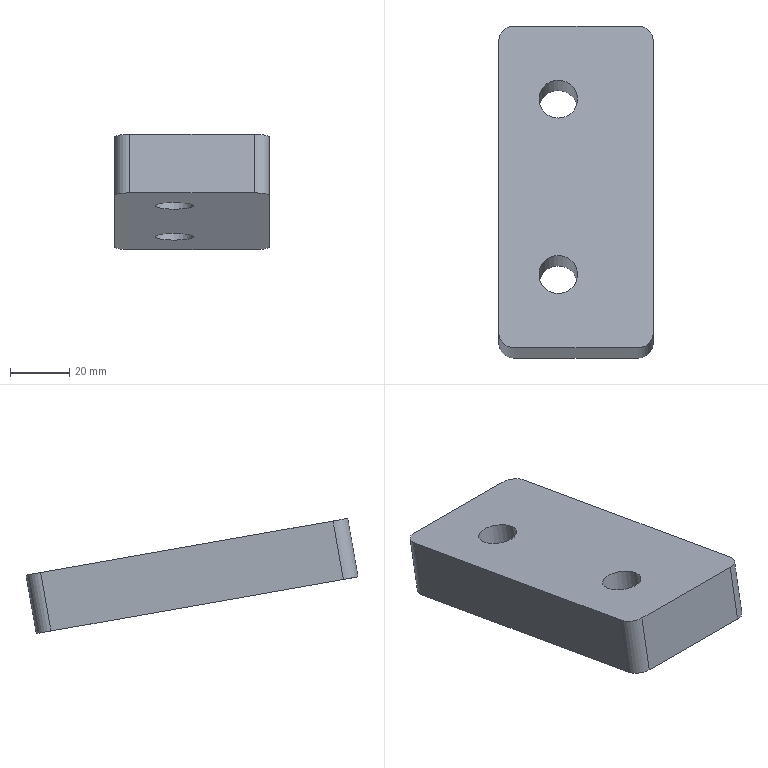Part | NX | features MAIN_BODY 2 | 1 solid | 12 faces | box 52 x 111.802 x 38.797 mm | volume 108662 mm3 | plane 6 | cylinder 6 | commonest cylinder face diameters 10 x4 13 x2
STEP:
#1=CARTESIAN_POINT('',(-1300.762,-795.713,-43.014));
#2=VERTEX_POINT('',#1);
#3=CARTESIAN_POINT('',(-1342.762,-795.713,-43.014));
#4=VERTEX_POINT('',#3);
#5=CARTESIAN_POINT('',(-1295.762,-795.713,-43.014));
#6=DIRECTION('',(-1.,0.,0.));
#7=VECTOR('',#6,1000.);
#8=LINE('',#5,#7);
#9=EDGE_CURVE('',#2,#4,#8,.T.);
#10=ORIENTED_EDGE('',*,*,#9,.T.);
#11=CARTESIAN_POINT('',(-1342.762,-792.24,-23.318));
#12=VERTEX_POINT('',#11);
#13=CARTESIAN_POINT('',(-1342.762,-792.24,-23.318));
#14=DIRECTION('',(0.,-0.1736,-0.9848));
#15=VECTOR('',#14,1000.);
#16=LINE('',#13,#15);
#17=EDGE_CURVE('',#12,#4,#16,.T.);
#18=ORIENTED_EDGE('',*,*,#17,.F.);
#19=CARTESIAN_POINT('',(-1300.762,-792.24,-23.318));
#20=VERTEX_POINT('',#19);
#21=CARTESIAN_POINT('',(-1295.762,-792.24,-23.318));
#22=DIRECTION('',(-1.,0.,0.));
#23=VECTOR('',#22,1000.);
#24=LINE('',#21,#23);
#25=EDGE_CURVE('',#20,#12,#24,.T.);
#26=ORIENTED_EDGE('',*,*,#25,.F.);
#27=CARTESIAN_POINT('',(-1300.762,-792.24,-23.318));
#28=DIRECTION('',(0.,-0.1736,-0.9848));
#29=VECTOR('',#28,1000.);
#30=LINE('',#27,#29);
#31=EDGE_CURVE('',#2,#20,#30,.F.);
#32=ORIENTED_EDGE('',*,*,#31,.F.);
#33=EDGE_LOOP('',(#10,#18,#26,#32));
#34=FACE_BOUND('',#33,.T.);
#35=CARTESIAN_POINT('',(-1295.762,-792.24,-23.318));
#36=DIRECTION('',(0.,0.9848,-0.1736));
#37=DIRECTION('',(1.,0.,0.));
#38=AXIS2_PLACEMENT_3D('',#35,#36,#37);
#39=PLANE('',#38);
#40=ADVANCED_FACE('',(#34),#39,.T.);
#41=CARTESIAN_POINT('',(-1347.762,-800.637,-42.145));
#42=VERTEX_POINT('',#41);
#43=CARTESIAN_POINT('',(-1347.762,-899.118,-24.781));
#44=VERTEX_POINT('',#43);
#45=CARTESIAN_POINT('',(-1347.762,-795.713,-43.014));
#46=DIRECTION('',(0.,-0.9848,0.1736));
#47=VECTOR('',#46,1000.);
#48=LINE('',#45,#47);
#49=EDGE_CURVE('',#42,#44,#48,.T.);
#50=ORIENTED_EDGE('',*,*,#49,.T.);
#51=CARTESIAN_POINT('',(-1347.762,-895.645,-5.085));
#52=VERTEX_POINT('',#51);
#53=CARTESIAN_POINT('',(-1347.762,-895.645,-5.085));
#54=DIRECTION('',(0.,-0.1736,-0.9848));
#55=VECTOR('',#54,1000.);
#56=LINE('',#53,#55);
#57=EDGE_CURVE('',#52,#44,#56,.T.);
#58=ORIENTED_EDGE('',*,*,#57,.F.);
#59=CARTESIAN_POINT('',(-1347.762,-797.164,-22.449));
#60=VERTEX_POINT('',#59);
#61=CARTESIAN_POINT('',(-1347.762,-792.24,-23.318));
#62=DIRECTION('',(0.,-0.9848,0.1736));
#63=VECTOR('',#62,1000.);
#64=LINE('',#61,#63);
#65=EDGE_CURVE('',#60,#52,#64,.T.);
#66=ORIENTED_EDGE('',*,*,#65,.F.);
#67=CARTESIAN_POINT('',(-1347.762,-797.164,-22.449));
#68=DIRECTION('',(0.,-0.1736,-0.9848));
#69=VECTOR('',#68,1000.);
#70=LINE('',#67,#69);
#71=EDGE_CURVE('',#42,#60,#70,.F.);
#72=ORIENTED_EDGE('',*,*,#71,.F.);
#73=EDGE_LOOP('',(#50,#58,#66,#72));
#74=FACE_BOUND('',#73,.T.);
#75=CARTESIAN_POINT('',(-1347.762,-792.24,-23.318));
#76=DIRECTION('',(-1.,0.,0.));
#77=DIRECTION('',(0.,0.9848,-0.1736));
#78=AXIS2_PLACEMENT_3D('',#75,#76,#77);
#79=PLANE('',#78);
#80=ADVANCED_FACE('',(#74),#79,.T.);
#81=CARTESIAN_POINT('',(-1295.762,-895.645,-5.085));
#82=VERTEX_POINT('',#81);
#83=CARTESIAN_POINT('',(-1295.762,-797.164,-22.449));
#84=VERTEX_POINT('',#83);
#85=CARTESIAN_POINT('',(-1295.762,-866.101,-10.294));
#86=DIRECTION('',(0.,0.9848,-0.1736));
#87=VECTOR('',#86,1000.);
#88=LINE('',#85,#87);
#89=EDGE_CURVE('',#82,#84,#88,.T.);
#90=ORIENTED_EDGE('',*,*,#89,.F.);
#91=CARTESIAN_POINT('',(-1295.762,-899.118,-24.781));
#92=VERTEX_POINT('',#91);
#93=CARTESIAN_POINT('',(-1295.762,-895.645,-5.085));
#94=DIRECTION('',(0.,-0.1736,-0.9848));
#95=VECTOR('',#94,1000.);
#96=LINE('',#93,#95);
#97=EDGE_CURVE('',#92,#82,#96,.F.);
#98=ORIENTED_EDGE('',*,*,#97,.F.);
#99=CARTESIAN_POINT('',(-1295.762,-800.637,-42.145));
#100=VERTEX_POINT('',#99);
#101=CARTESIAN_POINT('',(-1295.762,-869.574,-29.99));
#102=DIRECTION('',(0.,0.9848,-0.1736));
#103=VECTOR('',#102,1000.);
#104=LINE('',#101,#103);
#105=EDGE_CURVE('',#92,#100,#104,.T.);
#106=ORIENTED_EDGE('',*,*,#105,.T.);
#107=CARTESIAN_POINT('',(-1295.762,-797.164,-22.449));
#108=DIRECTION('',(0.,-0.1736,-0.9848));
#109=VECTOR('',#108,1000.);
#110=LINE('',#107,#109);
#111=EDGE_CURVE('',#84,#100,#110,.T.);
#112=ORIENTED_EDGE('',*,*,#111,.F.);
#113=EDGE_LOOP('',(#90,#98,#106,#112));
#114=FACE_BOUND('',#113,.T.);
#115=CARTESIAN_POINT('',(-1295.762,-866.101,-10.294));
#116=DIRECTION('',(1.,0.,0.));
#117=DIRECTION('',(0.,-0.9848,0.1736));
#118=AXIS2_PLACEMENT_3D('',#115,#116,#117);
#119=PLANE('',#118);
#120=ADVANCED_FACE('',(#114),#119,.T.);
#121=ORIENTED_EDGE('',*,*,#25,.T.);
#122=CARTESIAN_POINT('',(-1342.762,-797.164,-22.449));
#123=DIRECTION('',(0.,0.1736,0.9848));
#124=DIRECTION('',(0.,-0.9848,0.1736));
#125=AXIS2_PLACEMENT_3D('',#122,#123,#124);
#126=CIRCLE('',#125,5.);
#127=EDGE_CURVE('',#60,#12,#126,.F.);
#128=ORIENTED_EDGE('',*,*,#127,.F.);
#129=ORIENTED_EDGE('',*,*,#65,.T.);
#130=CARTESIAN_POINT('',(-1342.762,-900.569,-4.216));
#131=VERTEX_POINT('',#130);
#132=CARTESIAN_POINT('',(-1342.762,-895.645,-5.085));
#133=DIRECTION('',(0.,0.1736,0.9848));
#134=DIRECTION('',(0.,-0.9848,0.1736));
#135=AXIS2_PLACEMENT_3D('',#132,#133,#134);
#136=CIRCLE('',#135,5.);
#137=EDGE_CURVE('',#131,#52,#136,.F.);
#138=ORIENTED_EDGE('',*,*,#137,.F.);
#139=CARTESIAN_POINT('',(-1300.762,-900.569,-4.216));
#140=VERTEX_POINT('',#139);
#141=CARTESIAN_POINT('',(-1295.762,-900.569,-4.216));
#142=DIRECTION('',(-1.,0.,0.));
#143=VECTOR('',#142,1000.);
#144=LINE('',#141,#143);
#145=EDGE_CURVE('',#140,#131,#144,.T.);
#146=ORIENTED_EDGE('',*,*,#145,.F.);
#147=CARTESIAN_POINT('',(-1300.762,-895.645,-5.085));
#148=DIRECTION('',(0.,0.1736,0.9848));
#149=DIRECTION('',(0.,-0.9848,0.1736));
#150=AXIS2_PLACEMENT_3D('',#147,#148,#149);
#151=CIRCLE('',#150,5.);
#152=EDGE_CURVE('',#82,#140,#151,.F.);
#153=ORIENTED_EDGE('',*,*,#152,.F.);
#154=ORIENTED_EDGE('',*,*,#89,.T.);
#155=CARTESIAN_POINT('',(-1300.762,-797.164,-22.449));
#156=DIRECTION('',(0.,0.1736,0.9848));
#157=DIRECTION('',(0.,-0.9848,0.1736));
#158=AXIS2_PLACEMENT_3D('',#155,#156,#157);
#159=CIRCLE('',#158,5.);
#160=EDGE_CURVE('',#20,#84,#159,.F.);
#161=ORIENTED_EDGE('',*,*,#160,.F.);
#162=EDGE_LOOP('',(#121,#128,#129,#138,#146,#153,#154,#161));
#163=FACE_BOUND('',#162,.T.);
#164=CARTESIAN_POINT('',(-1327.762,-823.262,-17.848));
#165=VERTEX_POINT('',#164);
#166=CARTESIAN_POINT('',(-1327.762,-816.861,-18.976));
#167=DIRECTION('',(0.,0.1736,0.9848));
#168=DIRECTION('',(0.,-0.9848,0.1736));
#169=AXIS2_PLACEMENT_3D('',#166,#167,#168);
#170=CIRCLE('',#169,6.5);
#171=EDGE_CURVE('',#165,#165,#170,.T.);
#172=ORIENTED_EDGE('',*,*,#171,.F.);
#173=EDGE_LOOP('',(#172));
#174=FACE_BOUND('',#173,.T.);
#175=CARTESIAN_POINT('',(-1327.762,-882.35,-7.429));
#176=VERTEX_POINT('',#175);
#177=CARTESIAN_POINT('',(-1327.762,-875.949,-8.557));
#178=DIRECTION('',(0.,0.1736,0.9848));
#179=DIRECTION('',(0.,-0.9848,0.1736));
#180=AXIS2_PLACEMENT_3D('',#177,#178,#179);
#181=CIRCLE('',#180,6.5);
#182=EDGE_CURVE('',#176,#176,#181,.T.);
#183=ORIENTED_EDGE('',*,*,#182,.F.);
#184=EDGE_LOOP('',(#183));
#185=FACE_BOUND('',#184,.T.);
#186=CARTESIAN_POINT('',(-1347.762,-792.24,-23.318));
#187=DIRECTION('',(0.,-0.1736,-0.9848));
#188=DIRECTION('',(0.,-0.9848,0.1736));
#189=AXIS2_PLACEMENT_3D('',#186,#187,#188);
#190=PLANE('',#189);
#191=ADVANCED_FACE('',(#163,#174,#185),#190,.F.);
#192=ORIENTED_EDGE('',*,*,#105,.F.);
#193=CARTESIAN_POINT('',(-1300.762,-904.042,-23.912));
#194=VERTEX_POINT('',#193);
#195=CARTESIAN_POINT('',(-1300.762,-899.118,-24.781));
#196=DIRECTION('',(0.,0.1736,0.9848));
#197=DIRECTION('',(0.,-0.9848,0.1736));
#198=AXIS2_PLACEMENT_3D('',#195,#196,#197);
#199=CIRCLE('',#198,5.);
#200=EDGE_CURVE('',#194,#92,#199,.T.);
#201=ORIENTED_EDGE('',*,*,#200,.F.);
#202=CARTESIAN_POINT('',(-1342.762,-904.042,-23.912));
#203=VERTEX_POINT('',#202);
#204=CARTESIAN_POINT('',(-1295.762,-904.042,-23.912));
#205=DIRECTION('',(-1.,0.,0.));
#206=VECTOR('',#205,1000.);
#207=LINE('',#204,#206);
#208=EDGE_CURVE('',#194,#203,#207,.T.);
#209=ORIENTED_EDGE('',*,*,#208,.T.);
#210=CARTESIAN_POINT('',(-1342.762,-899.118,-24.781));
#211=DIRECTION('',(0.,0.1736,0.9848));
#212=DIRECTION('',(0.,-0.9848,0.1736));
#213=AXIS2_PLACEMENT_3D('',#210,#211,#212);
#214=CIRCLE('',#213,5.);
#215=EDGE_CURVE('',#44,#203,#214,.T.);
#216=ORIENTED_EDGE('',*,*,#215,.F.);
#217=ORIENTED_EDGE('',*,*,#49,.F.);
#218=CARTESIAN_POINT('',(-1342.762,-800.637,-42.145));
#219=DIRECTION('',(0.,0.1736,0.9848));
#220=DIRECTION('',(0.,-0.9848,0.1736));
#221=AXIS2_PLACEMENT_3D('',#218,#219,#220);
#222=CIRCLE('',#221,5.);
#223=EDGE_CURVE('',#4,#42,#222,.T.);
#224=ORIENTED_EDGE('',*,*,#223,.F.);
#225=ORIENTED_EDGE('',*,*,#9,.F.);
#226=CARTESIAN_POINT('',(-1300.762,-800.637,-42.145));
#227=DIRECTION('',(0.,0.1736,0.9848));
#228=DIRECTION('',(0.,-0.9848,0.1736));
#229=AXIS2_PLACEMENT_3D('',#226,#227,#228);
#230=CIRCLE('',#229,5.);
#231=EDGE_CURVE('',#100,#2,#230,.T.);
#232=ORIENTED_EDGE('',*,*,#231,.F.);
#233=EDGE_LOOP('',(#192,#201,#209,#216,#217,#224,#225,#232));
#234=FACE_BOUND('',#233,.T.);
#235=CARTESIAN_POINT('',(-1327.762,-885.823,-27.125));
#236=VERTEX_POINT('',#235);
#237=CARTESIAN_POINT('',(-1327.762,-879.422,-28.254));
#238=DIRECTION('',(0.,0.1736,0.9848));
#239=DIRECTION('',(0.,-0.9848,0.1736));
#240=AXIS2_PLACEMENT_3D('',#237,#238,#239);
#241=CIRCLE('',#240,6.5);
#242=EDGE_CURVE('',#236,#236,#241,.T.);
#243=ORIENTED_EDGE('',*,*,#242,.T.);
#244=EDGE_LOOP('',(#243));
#245=FACE_BOUND('',#244,.T.);
#246=CARTESIAN_POINT('',(-1327.762,-826.735,-37.544));
#247=VERTEX_POINT('',#246);
#248=CARTESIAN_POINT('',(-1327.762,-820.334,-38.673));
#249=DIRECTION('',(0.,0.1736,0.9848));
#250=DIRECTION('',(0.,-0.9848,0.1736));
#251=AXIS2_PLACEMENT_3D('',#248,#249,#250);
#252=CIRCLE('',#251,6.5);
#253=EDGE_CURVE('',#247,#247,#252,.T.);
#254=ORIENTED_EDGE('',*,*,#253,.T.);
#255=EDGE_LOOP('',(#254));
#256=FACE_BOUND('',#255,.T.);
#257=CARTESIAN_POINT('',(-1347.762,-795.713,-43.014));
#258=DIRECTION('',(0.,-0.1736,-0.9848));
#259=DIRECTION('',(0.,-0.9848,0.1736));
#260=AXIS2_PLACEMENT_3D('',#257,#258,#259);
#261=PLANE('',#260);
#262=ADVANCED_FACE('',(#234,#245,#256),#261,.T.);
#263=ORIENTED_EDGE('',*,*,#253,.F.);
#264=EDGE_LOOP('',(#263));
#265=FACE_BOUND('',#264,.T.);
#266=ORIENTED_EDGE('',*,*,#171,.T.);
#267=EDGE_LOOP('',(#266));
#268=FACE_BOUND('',#267,.T.);
#269=CARTESIAN_POINT('',(-1327.762,-816.861,-18.976));
#270=DIRECTION('',(0.,-0.1736,-0.9848));
#271=DIRECTION('',(0.,-0.9848,0.1736));
#272=AXIS2_PLACEMENT_3D('',#269,#270,#271);
#273=CYLINDRICAL_SURFACE('',#272,6.5);
#274=ADVANCED_FACE('',(#265,#268),#273,.F.);
#275=ORIENTED_EDGE('',*,*,#242,.F.);
#276=EDGE_LOOP('',(#275));
#277=FACE_BOUND('',#276,.T.);
#278=ORIENTED_EDGE('',*,*,#182,.T.);
#279=EDGE_LOOP('',(#278));
#280=FACE_BOUND('',#279,.T.);
#281=CARTESIAN_POINT('',(-1327.762,-875.949,-8.557));
#282=DIRECTION('',(0.,-0.1736,-0.9848));
#283=DIRECTION('',(0.,-0.9848,0.1736));
#284=AXIS2_PLACEMENT_3D('',#281,#282,#283);
#285=CYLINDRICAL_SURFACE('',#284,6.5);
#286=ADVANCED_FACE('',(#277,#280),#285,.F.);
#287=ORIENTED_EDGE('',*,*,#145,.T.);
#288=CARTESIAN_POINT('',(-1342.762,-900.569,-4.216));
#289=DIRECTION('',(0.,-0.1736,-0.9848));
#290=VECTOR('',#289,1000.);
#291=LINE('',#288,#290);
#292=EDGE_CURVE('',#203,#131,#291,.F.);
#293=ORIENTED_EDGE('',*,*,#292,.F.);
#294=ORIENTED_EDGE('',*,*,#208,.F.);
#295=CARTESIAN_POINT('',(-1300.762,-900.569,-4.216));
#296=DIRECTION('',(0.,-0.1736,-0.9848));
#297=VECTOR('',#296,1000.);
#298=LINE('',#295,#297);
#299=EDGE_CURVE('',#140,#194,#298,.T.);
#300=ORIENTED_EDGE('',*,*,#299,.F.);
#301=EDGE_LOOP('',(#287,#293,#294,#300));
#302=FACE_BOUND('',#301,.T.);
#303=CARTESIAN_POINT('',(-1295.762,-900.569,-4.216));
#304=DIRECTION('',(0.,-0.9848,0.1736));
#305=DIRECTION('',(1.,0.,0.));
#306=AXIS2_PLACEMENT_3D('',#303,#304,#305);
#307=PLANE('',#306);
#308=ADVANCED_FACE('',(#302),#307,.T.);
#309=ORIENTED_EDGE('',*,*,#160,.T.);
#310=ORIENTED_EDGE('',*,*,#111,.T.);
#311=ORIENTED_EDGE('',*,*,#231,.T.);
#312=ORIENTED_EDGE('',*,*,#31,.T.);
#313=EDGE_LOOP('',(#309,#310,#311,#312));
#314=FACE_BOUND('',#313,.T.);
#315=CARTESIAN_POINT('',(-1300.762,-797.164,-22.449));
#316=DIRECTION('',(0.,-0.1736,-0.9848));
#317=DIRECTION('',(0.,-0.9848,0.1736));
#318=AXIS2_PLACEMENT_3D('',#315,#316,#317);
#319=CYLINDRICAL_SURFACE('',#318,5.);
#320=ADVANCED_FACE('',(#314),#319,.T.);
#321=ORIENTED_EDGE('',*,*,#127,.T.);
#322=ORIENTED_EDGE('',*,*,#17,.T.);
#323=ORIENTED_EDGE('',*,*,#223,.T.);
#324=ORIENTED_EDGE('',*,*,#71,.T.);
#325=EDGE_LOOP('',(#321,#322,#323,#324));
#326=FACE_BOUND('',#325,.T.);
#327=CARTESIAN_POINT('',(-1342.762,-797.164,-22.449));
#328=DIRECTION('',(0.,-0.1736,-0.9848));
#329=DIRECTION('',(0.,-0.9848,0.1736));
#330=AXIS2_PLACEMENT_3D('',#327,#328,#329);
#331=CYLINDRICAL_SURFACE('',#330,5.);
#332=ADVANCED_FACE('',(#326),#331,.T.);
#333=ORIENTED_EDGE('',*,*,#152,.T.);
#334=ORIENTED_EDGE('',*,*,#299,.T.);
#335=ORIENTED_EDGE('',*,*,#200,.T.);
#336=ORIENTED_EDGE('',*,*,#97,.T.);
#337=EDGE_LOOP('',(#333,#334,#335,#336));
#338=FACE_BOUND('',#337,.T.);
#339=CARTESIAN_POINT('',(-1300.762,-895.645,-5.085));
#340=DIRECTION('',(0.,-0.1736,-0.9848));
#341=DIRECTION('',(0.,-0.9848,0.1736));
#342=AXIS2_PLACEMENT_3D('',#339,#340,#341);
#343=CYLINDRICAL_SURFACE('',#342,5.);
#344=ADVANCED_FACE('',(#338),#343,.T.);
#345=ORIENTED_EDGE('',*,*,#137,.T.);
#346=ORIENTED_EDGE('',*,*,#57,.T.);
#347=ORIENTED_EDGE('',*,*,#215,.T.);
#348=ORIENTED_EDGE('',*,*,#292,.T.);
#349=EDGE_LOOP('',(#345,#346,#347,#348));
#350=FACE_BOUND('',#349,.T.);
#351=CARTESIAN_POINT('',(-1342.762,-895.645,-5.085));
#352=DIRECTION('',(0.,-0.1736,-0.9848));
#353=DIRECTION('',(0.,-0.9848,0.1736));
#354=AXIS2_PLACEMENT_3D('',#351,#352,#353);
#355=CYLINDRICAL_SURFACE('',#354,5.);
#356=ADVANCED_FACE('',(#350),#355,.T.);
#357=CLOSED_SHELL('',(#40,#80,#120,#191,#262,#274,#286,#308,#320,#332,#344,#356));
#358=MANIFOLD_SOLID_BREP('',#357);
#359=(LENGTH_UNIT()NAMED_UNIT(*)SI_UNIT(.MILLI.,.METRE.));
#360=UNCERTAINTY_MEASURE_WITH_UNIT(LENGTH_MEASURE(0.00001),#359,'','');
#361=(NAMED_UNIT(*)PLANE_ANGLE_UNIT()SI_UNIT($,.RADIAN.));
#362=(NAMED_UNIT(*)SI_UNIT($,.STERADIAN.)SOLID_ANGLE_UNIT());
#363=(GEOMETRIC_REPRESENTATION_CONTEXT(3)GLOBAL_UNCERTAINTY_ASSIGNED_CONTEXT((#360))GLOBAL_UNIT_ASSIGNED_CONTEXT((#359,#361,#362))REPRESENTATION_CONTEXT('',''));
#364=ADVANCED_BREP_SHAPE_REPRESENTATION('',(#358),#363);